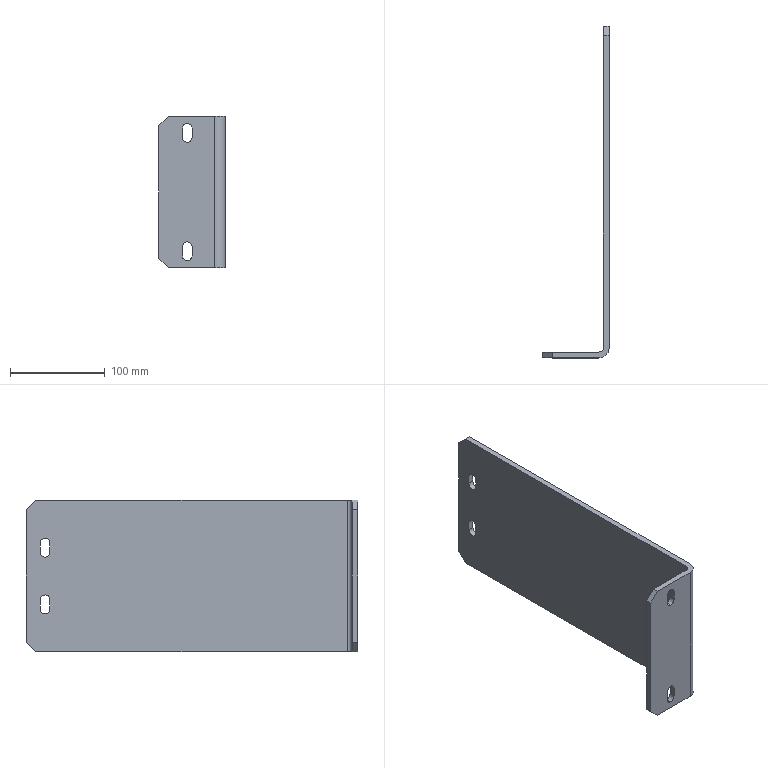Part | STEP file | VD-SYL0380DJ1006_1-1_VD-SYL0380 | 1 solid | 34 faces | box 70 x 350 x 160 mm | volume 388659 mm3 | plane 20 | cylinder 14 | commonest cylinder face diameters 10 x13 22 x1
STEP:
#1=CARTESIAN_POINT('',(0.,325.,35.));
#2=VERTEX_POINT('',#1);
#3=CARTESIAN_POINT('',(0.,330.,40.));
#4=VERTEX_POINT('',#3);
#5=CARTESIAN_POINT('',(0.,330.,35.));
#6=DIRECTION('',(-1.,0.,0.));
#7=DIRECTION('',(0.,-1.,0.));
#8=AXIS2_PLACEMENT_3D('',#5,#6,#7);
#9=CIRCLE('',#8,5.);
#10=EDGE_CURVE('',#2,#4,#9,.T.);
#11=ORIENTED_EDGE('',*,*,#10,.F.);
#12=CARTESIAN_POINT('',(-6.,325.,35.));
#13=VERTEX_POINT('',#12);
#14=CARTESIAN_POINT('',(0.,325.,35.));
#15=DIRECTION('',(-1.,0.,0.));
#16=VECTOR('',#15,1000.);
#17=LINE('',#14,#16);
#18=EDGE_CURVE('',#2,#13,#17,.T.);
#19=ORIENTED_EDGE('',*,*,#18,.T.);
#20=CARTESIAN_POINT('',(-6.,330.,40.));
#21=VERTEX_POINT('',#20);
#22=CARTESIAN_POINT('',(-6.,330.,35.));
#23=DIRECTION('',(1.,0.,0.));
#24=DIRECTION('',(0.,0.,1.));
#25=AXIS2_PLACEMENT_3D('',#22,#23,#24);
#26=CIRCLE('',#25,5.);
#27=EDGE_CURVE('',#21,#13,#26,.T.);
#28=ORIENTED_EDGE('',*,*,#27,.F.);
#29=CARTESIAN_POINT('',(-6.,330.,40.));
#30=DIRECTION('',(1.,0.,0.));
#31=VECTOR('',#30,1000.);
#32=LINE('',#29,#31);
#33=EDGE_CURVE('',#21,#4,#32,.T.);
#34=ORIENTED_EDGE('',*,*,#33,.T.);
#35=EDGE_LOOP('',(#11,#19,#28,#34));
#36=FACE_OUTER_BOUND('',#35,.T.);
#37=CARTESIAN_POINT('',(-3.,330.,35.));
#38=DIRECTION('',(-1.,0.,0.));
#39=DIRECTION('',(0.,0.,1.));
#40=AXIS2_PLACEMENT_3D('',#37,#38,#39);
#41=CYLINDRICAL_SURFACE('',#40,5.);
#42=ADVANCED_FACE('',(#36),#41,.F.);
#43=ORIENTED_EDGE('',*,*,#33,.F.);
#44=CARTESIAN_POINT('',(-6.,335.,35.));
#45=VERTEX_POINT('',#44);
#46=CARTESIAN_POINT('',(-6.,330.,35.));
#47=DIRECTION('',(1.,0.,0.));
#48=DIRECTION('',(0.,1.,0.));
#49=AXIS2_PLACEMENT_3D('',#46,#47,#48);
#50=CIRCLE('',#49,5.);
#51=EDGE_CURVE('',#45,#21,#50,.T.);
#52=ORIENTED_EDGE('',*,*,#51,.F.);
#53=CARTESIAN_POINT('',(0.,335.,35.));
#54=VERTEX_POINT('',#53);
#55=CARTESIAN_POINT('',(-6.,335.,35.));
#56=DIRECTION('',(1.,0.,0.));
#57=VECTOR('',#56,1000.);
#58=LINE('',#55,#57);
#59=EDGE_CURVE('',#45,#54,#58,.T.);
#60=ORIENTED_EDGE('',*,*,#59,.T.);
#61=CARTESIAN_POINT('',(0.,330.,35.));
#62=DIRECTION('',(-1.,0.,0.));
#63=DIRECTION('',(0.,0.,1.));
#64=AXIS2_PLACEMENT_3D('',#61,#62,#63);
#65=CIRCLE('',#64,5.);
#66=EDGE_CURVE('',#4,#54,#65,.T.);
#67=ORIENTED_EDGE('',*,*,#66,.F.);
#68=EDGE_LOOP('',(#43,#52,#60,#67));
#69=FACE_OUTER_BOUND('',#68,.T.);
#70=CARTESIAN_POINT('',(-3.,330.,35.));
#71=DIRECTION('',(-1.,0.,0.));
#72=DIRECTION('',(0.,0.,1.));
#73=AXIS2_PLACEMENT_3D('',#70,#71,#72);
#74=CYLINDRICAL_SURFACE('',#73,5.);
#75=ADVANCED_FACE('',(#69),#74,.F.);
#76=CARTESIAN_POINT('',(0.,335.,25.));
#77=VERTEX_POINT('',#76);
#78=CARTESIAN_POINT('',(-6.,335.,25.));
#79=VERTEX_POINT('',#78);
#80=CARTESIAN_POINT('',(0.,335.,25.));
#81=DIRECTION('',(-1.,0.,0.));
#82=VECTOR('',#81,1000.);
#83=LINE('',#80,#82);
#84=EDGE_CURVE('',#77,#79,#83,.T.);
#85=ORIENTED_EDGE('',*,*,#84,.F.);
#86=CARTESIAN_POINT('',(0.,335.,25.));
#87=DIRECTION('',(0.,0.,1.));
#88=VECTOR('',#87,1000.);
#89=LINE('',#86,#88);
#90=EDGE_CURVE('',#77,#54,#89,.T.);
#91=ORIENTED_EDGE('',*,*,#90,.T.);
#92=ORIENTED_EDGE('',*,*,#59,.F.);
#93=CARTESIAN_POINT('',(-6.,335.,25.));
#94=DIRECTION('',(0.,0.,1.));
#95=VECTOR('',#94,1000.);
#96=LINE('',#93,#95);
#97=EDGE_CURVE('',#79,#45,#96,.T.);
#98=ORIENTED_EDGE('',*,*,#97,.F.);
#99=EDGE_LOOP('',(#85,#91,#92,#98));
#100=FACE_OUTER_BOUND('',#99,.T.);
#101=CARTESIAN_POINT('',(-3.,335.,30.));
#102=DIRECTION('',(0.,1.,0.));
#103=DIRECTION('',(1.,0.,0.));
#104=AXIS2_PLACEMENT_3D('',#101,#102,#103);
#105=PLANE('',#104);
#106=ADVANCED_FACE('',(#100),#105,.F.);
#107=CARTESIAN_POINT('',(-6.,325.,25.));
#108=VERTEX_POINT('',#107);
#109=CARTESIAN_POINT('',(-6.,330.,25.));
#110=DIRECTION('',(1.,0.,0.));
#111=DIRECTION('',(0.,0.,-1.));
#112=AXIS2_PLACEMENT_3D('',#109,#110,#111);
#113=CIRCLE('',#112,5.);
#114=EDGE_CURVE('',#108,#79,#113,.T.);
#115=ORIENTED_EDGE('',*,*,#114,.F.);
#116=CARTESIAN_POINT('',(0.,325.,25.));
#117=VERTEX_POINT('',#116);
#118=CARTESIAN_POINT('',(-6.,325.,25.));
#119=DIRECTION('',(1.,0.,0.));
#120=VECTOR('',#119,1000.);
#121=LINE('',#118,#120);
#122=EDGE_CURVE('',#108,#117,#121,.T.);
#123=ORIENTED_EDGE('',*,*,#122,.T.);
#124=CARTESIAN_POINT('',(0.,330.,25.));
#125=DIRECTION('',(-1.,0.,0.));
#126=DIRECTION('',(0.,1.,0.));
#127=AXIS2_PLACEMENT_3D('',#124,#125,#126);
#128=CIRCLE('',#127,5.);
#129=EDGE_CURVE('',#77,#117,#128,.T.);
#130=ORIENTED_EDGE('',*,*,#129,.F.);
#131=ORIENTED_EDGE('',*,*,#84,.T.);
#132=EDGE_LOOP('',(#115,#123,#130,#131));
#133=FACE_OUTER_BOUND('',#132,.T.);
#134=CARTESIAN_POINT('',(-3.,330.,25.));
#135=DIRECTION('',(-1.,0.,0.));
#136=DIRECTION('',(0.,0.,1.));
#137=AXIS2_PLACEMENT_3D('',#134,#135,#136);
#138=CYLINDRICAL_SURFACE('',#137,5.);
#139=ADVANCED_FACE('',(#133),#138,.F.);
#140=ORIENTED_EDGE('',*,*,#18,.F.);
#141=CARTESIAN_POINT('',(0.,325.,35.));
#142=DIRECTION('',(0.,0.,-1.));
#143=VECTOR('',#142,1000.);
#144=LINE('',#141,#143);
#145=EDGE_CURVE('',#2,#117,#144,.T.);
#146=ORIENTED_EDGE('',*,*,#145,.T.);
#147=ORIENTED_EDGE('',*,*,#122,.F.);
#148=CARTESIAN_POINT('',(-6.,325.,35.));
#149=DIRECTION('',(0.,0.,-1.));
#150=VECTOR('',#149,1000.);
#151=LINE('',#148,#150);
#152=EDGE_CURVE('',#13,#108,#151,.T.);
#153=ORIENTED_EDGE('',*,*,#152,.F.);
#154=EDGE_LOOP('',(#140,#146,#147,#153));
#155=FACE_OUTER_BOUND('',#154,.T.);
#156=CARTESIAN_POINT('',(-3.,325.,30.));
#157=DIRECTION('',(0.,-1.,0.));
#158=DIRECTION('',(0.,0.,-1.));
#159=AXIS2_PLACEMENT_3D('',#156,#157,#158);
#160=PLANE('',#159);
#161=ADVANCED_FACE('',(#155),#160,.F.);
#162=CARTESIAN_POINT('',(0.,325.,-25.));
#163=VERTEX_POINT('',#162);
#164=CARTESIAN_POINT('',(-6.,325.,-25.));
#165=VERTEX_POINT('',#164);
#166=CARTESIAN_POINT('',(0.,325.,-25.));
#167=DIRECTION('',(-1.,0.,0.));
#168=VECTOR('',#167,1000.);
#169=LINE('',#166,#168);
#170=EDGE_CURVE('',#163,#165,#169,.T.);
#171=ORIENTED_EDGE('',*,*,#170,.F.);
#172=CARTESIAN_POINT('',(0.,325.,-35.));
#173=VERTEX_POINT('',#172);
#174=CARTESIAN_POINT('',(0.,325.,-25.));
#175=DIRECTION('',(0.,0.,-1.));
#176=VECTOR('',#175,1000.);
#177=LINE('',#174,#176);
#178=EDGE_CURVE('',#163,#173,#177,.T.);
#179=ORIENTED_EDGE('',*,*,#178,.T.);
#180=CARTESIAN_POINT('',(-6.,325.,-35.));
#181=VERTEX_POINT('',#180);
#182=CARTESIAN_POINT('',(-6.,325.,-35.));
#183=DIRECTION('',(1.,0.,0.));
#184=VECTOR('',#183,1000.);
#185=LINE('',#182,#184);
#186=EDGE_CURVE('',#181,#173,#185,.T.);
#187=ORIENTED_EDGE('',*,*,#186,.F.);
#188=CARTESIAN_POINT('',(-6.,325.,-25.));
#189=DIRECTION('',(0.,0.,-1.));
#190=VECTOR('',#189,1000.);
#191=LINE('',#188,#190);
#192=EDGE_CURVE('',#165,#181,#191,.T.);
#193=ORIENTED_EDGE('',*,*,#192,.F.);
#194=EDGE_LOOP('',(#171,#179,#187,#193));
#195=FACE_OUTER_BOUND('',#194,.T.);
#196=CARTESIAN_POINT('',(-3.,325.,-30.));
#197=DIRECTION('',(0.,-1.,0.));
#198=DIRECTION('',(0.,0.,-1.));
#199=AXIS2_PLACEMENT_3D('',#196,#197,#198);
#200=PLANE('',#199);
#201=ADVANCED_FACE('',(#195),#200,.F.);
#202=CARTESIAN_POINT('',(-6.,335.,-35.));
#203=VERTEX_POINT('',#202);
#204=CARTESIAN_POINT('',(-6.,330.,-35.));
#205=DIRECTION('',(1.,0.,0.));
#206=DIRECTION('',(0.,-1.,0.));
#207=AXIS2_PLACEMENT_3D('',#204,#205,#206);
#208=CIRCLE('',#207,5.);
#209=EDGE_CURVE('',#181,#203,#208,.T.);
#210=ORIENTED_EDGE('',*,*,#209,.F.);
#211=ORIENTED_EDGE('',*,*,#186,.T.);
#212=CARTESIAN_POINT('',(0.,335.,-35.));
#213=VERTEX_POINT('',#212);
#214=CARTESIAN_POINT('',(0.,330.,-35.));
#215=DIRECTION('',(-1.,0.,0.));
#216=DIRECTION('',(0.,1.,0.));
#217=AXIS2_PLACEMENT_3D('',#214,#215,#216);
#218=CIRCLE('',#217,5.);
#219=EDGE_CURVE('',#213,#173,#218,.T.);
#220=ORIENTED_EDGE('',*,*,#219,.F.);
#221=CARTESIAN_POINT('',(0.,335.,-35.));
#222=DIRECTION('',(-1.,0.,0.));
#223=VECTOR('',#222,1000.);
#224=LINE('',#221,#223);
#225=EDGE_CURVE('',#213,#203,#224,.T.);
#226=ORIENTED_EDGE('',*,*,#225,.T.);
#227=EDGE_LOOP('',(#210,#211,#220,#226));
#228=FACE_OUTER_BOUND('',#227,.T.);
#229=CARTESIAN_POINT('',(-3.,330.,-35.));
#230=DIRECTION('',(-1.,0.,0.));
#231=DIRECTION('',(0.,0.,1.));
#232=AXIS2_PLACEMENT_3D('',#229,#230,#231);
#233=CYLINDRICAL_SURFACE('',#232,5.);
#234=ADVANCED_FACE('',(#228),#233,.F.);
#235=ORIENTED_EDGE('',*,*,#225,.F.);
#236=CARTESIAN_POINT('',(0.,335.,-25.));
#237=VERTEX_POINT('',#236);
#238=CARTESIAN_POINT('',(0.,335.,-35.));
#239=DIRECTION('',(0.,0.,1.));
#240=VECTOR('',#239,1000.);
#241=LINE('',#238,#240);
#242=EDGE_CURVE('',#213,#237,#241,.T.);
#243=ORIENTED_EDGE('',*,*,#242,.T.);
#244=CARTESIAN_POINT('',(-6.,335.,-25.));
#245=VERTEX_POINT('',#244);
#246=CARTESIAN_POINT('',(-6.,335.,-25.));
#247=DIRECTION('',(1.,0.,0.));
#248=VECTOR('',#247,1000.);
#249=LINE('',#246,#248);
#250=EDGE_CURVE('',#245,#237,#249,.T.);
#251=ORIENTED_EDGE('',*,*,#250,.F.);
#252=CARTESIAN_POINT('',(-6.,335.,-35.));
#253=DIRECTION('',(0.,0.,1.));
#254=VECTOR('',#253,1000.);
#255=LINE('',#252,#254);
#256=EDGE_CURVE('',#203,#245,#255,.T.);
#257=ORIENTED_EDGE('',*,*,#256,.F.);
#258=EDGE_LOOP('',(#235,#243,#251,#257));
#259=FACE_OUTER_BOUND('',#258,.T.);
#260=CARTESIAN_POINT('',(-3.,335.,-30.));
#261=DIRECTION('',(0.,1.,0.));
#262=DIRECTION('',(1.,0.,0.));
#263=AXIS2_PLACEMENT_3D('',#260,#261,#262);
#264=PLANE('',#263);
#265=ADVANCED_FACE('',(#259),#264,.F.);
#266=CARTESIAN_POINT('',(-6.,330.,-20.));
#267=VERTEX_POINT('',#266);
#268=CARTESIAN_POINT('',(0.,330.,-20.));
#269=VERTEX_POINT('',#268);
#270=CARTESIAN_POINT('',(-6.,330.,-20.));
#271=DIRECTION('',(1.,0.,0.));
#272=VECTOR('',#271,1000.);
#273=LINE('',#270,#272);
#274=EDGE_CURVE('',#267,#269,#273,.T.);
#275=ORIENTED_EDGE('',*,*,#274,.F.);
#276=CARTESIAN_POINT('',(-6.,330.,-25.));
#277=DIRECTION('',(1.,0.,0.));
#278=DIRECTION('',(0.,1.,0.));
#279=AXIS2_PLACEMENT_3D('',#276,#277,#278);
#280=CIRCLE('',#279,5.);
#281=EDGE_CURVE('',#245,#267,#280,.T.);
#282=ORIENTED_EDGE('',*,*,#281,.F.);
#283=ORIENTED_EDGE('',*,*,#250,.T.);
#284=CARTESIAN_POINT('',(0.,330.,-25.));
#285=DIRECTION('',(-1.,0.,0.));
#286=DIRECTION('',(0.,0.,1.));
#287=AXIS2_PLACEMENT_3D('',#284,#285,#286);
#288=CIRCLE('',#287,5.);
#289=EDGE_CURVE('',#269,#237,#288,.T.);
#290=ORIENTED_EDGE('',*,*,#289,.F.);
#291=EDGE_LOOP('',(#275,#282,#283,#290));
#292=FACE_OUTER_BOUND('',#291,.T.);
#293=CARTESIAN_POINT('',(-3.,330.,-25.));
#294=DIRECTION('',(-1.,0.,0.));
#295=DIRECTION('',(0.,0.,1.));
#296=AXIS2_PLACEMENT_3D('',#293,#294,#295);
#297=CYLINDRICAL_SURFACE('',#296,5.);
#298=ADVANCED_FACE('',(#292),#297,.F.);
#299=CARTESIAN_POINT('',(0.,330.,-25.));
#300=DIRECTION('',(-1.,0.,0.));
#301=DIRECTION('',(0.,-1.,0.));
#302=AXIS2_PLACEMENT_3D('',#299,#300,#301);
#303=CIRCLE('',#302,5.);
#304=EDGE_CURVE('',#163,#269,#303,.T.);
#305=ORIENTED_EDGE('',*,*,#304,.F.);
#306=ORIENTED_EDGE('',*,*,#170,.T.);
#307=CARTESIAN_POINT('',(-6.,330.,-25.));
#308=DIRECTION('',(1.,0.,0.));
#309=DIRECTION('',(0.,0.,1.));
#310=AXIS2_PLACEMENT_3D('',#307,#308,#309);
#311=CIRCLE('',#310,5.);
#312=EDGE_CURVE('',#267,#165,#311,.T.);
#313=ORIENTED_EDGE('',*,*,#312,.F.);
#314=ORIENTED_EDGE('',*,*,#274,.T.);
#315=EDGE_LOOP('',(#305,#306,#313,#314));
#316=FACE_OUTER_BOUND('',#315,.T.);
#317=CARTESIAN_POINT('',(-3.,330.,-25.));
#318=DIRECTION('',(-1.,0.,0.));
#319=DIRECTION('',(0.,0.,1.));
#320=AXIS2_PLACEMENT_3D('',#317,#318,#319);
#321=CYLINDRICAL_SURFACE('',#320,5.);
#322=ADVANCED_FACE('',(#316),#321,.F.);
#323=CARTESIAN_POINT('',(0.,340.,-80.));
#324=VERTEX_POINT('',#323);
#325=CARTESIAN_POINT('',(0.,350.,-70.));
#326=VERTEX_POINT('',#325);
#327=CARTESIAN_POINT('',(0.,340.,-80.));
#328=DIRECTION('',(0.,0.7071,0.7071));
#329=VECTOR('',#328,1000.);
#330=LINE('',#327,#329);
#331=EDGE_CURVE('',#324,#326,#330,.T.);
#332=ORIENTED_EDGE('',*,*,#331,.F.);
#333=CARTESIAN_POINT('',(-6.,340.,-80.));
#334=VERTEX_POINT('',#333);
#335=CARTESIAN_POINT('',(0.,340.,-80.));
#336=DIRECTION('',(-1.,0.,0.));
#337=VECTOR('',#336,1000.);
#338=LINE('',#335,#337);
#339=EDGE_CURVE('',#324,#334,#338,.T.);
#340=ORIENTED_EDGE('',*,*,#339,.T.);
#341=CARTESIAN_POINT('',(-6.,350.,-70.));
#342=VERTEX_POINT('',#341);
#343=CARTESIAN_POINT('',(-6.,350.,-70.));
#344=DIRECTION('',(0.,-0.7071,-0.7071));
#345=VECTOR('',#344,1000.);
#346=LINE('',#343,#345);
#347=EDGE_CURVE('',#342,#334,#346,.T.);
#348=ORIENTED_EDGE('',*,*,#347,.F.);
#349=CARTESIAN_POINT('',(-6.,350.,-70.));
#350=DIRECTION('',(1.,0.,0.));
#351=VECTOR('',#350,1000.);
#352=LINE('',#349,#351);
#353=EDGE_CURVE('',#342,#326,#352,.T.);
#354=ORIENTED_EDGE('',*,*,#353,.T.);
#355=EDGE_LOOP('',(#332,#340,#348,#354));
#356=FACE_OUTER_BOUND('',#355,.T.);
#357=CARTESIAN_POINT('',(-3.,345.,-75.));
#358=DIRECTION('',(0.,0.7071,-0.7071));
#359=DIRECTION('',(-1.,0.,0.));
#360=AXIS2_PLACEMENT_3D('',#357,#358,#359);
#361=PLANE('',#360);
#362=ADVANCED_FACE('',(#356),#361,.T.);
#363=CARTESIAN_POINT('',(-45.,6.,57.5));
#364=VERTEX_POINT('',#363);
#365=CARTESIAN_POINT('',(-40.,6.,52.5));
#366=VERTEX_POINT('',#365);
#367=CARTESIAN_POINT('',(-40.,6.,57.5));
#368=DIRECTION('',(0.,-1.,0.));
#369=DIRECTION('',(-1.,0.,0.));
#370=AXIS2_PLACEMENT_3D('',#367,#368,#369);
#371=CIRCLE('',#370,5.);
#372=EDGE_CURVE('',#364,#366,#371,.T.);
#373=ORIENTED_EDGE('',*,*,#372,.F.);
#374=CARTESIAN_POINT('',(-45.,0.,57.5));
#375=VERTEX_POINT('',#374);
#376=CARTESIAN_POINT('',(-45.,6.,57.5));
#377=DIRECTION('',(0.,-1.,0.));
#378=VECTOR('',#377,1000.);
#379=LINE('',#376,#378);
#380=EDGE_CURVE('',#364,#375,#379,.T.);
#381=ORIENTED_EDGE('',*,*,#380,.T.);
#382=CARTESIAN_POINT('',(-40.,0.,52.5));
#383=VERTEX_POINT('',#382);
#384=CARTESIAN_POINT('',(-40.,0.,57.5));
#385=DIRECTION('',(0.,1.,0.));
#386=DIRECTION('',(0.,0.,-1.));
#387=AXIS2_PLACEMENT_3D('',#384,#385,#386);
#388=CIRCLE('',#387,5.);
#389=EDGE_CURVE('',#383,#375,#388,.T.);
#390=ORIENTED_EDGE('',*,*,#389,.F.);
#391=CARTESIAN_POINT('',(-40.,0.,52.5));
#392=DIRECTION('',(0.,1.,0.));
#393=VECTOR('',#392,1000.);
#394=LINE('',#391,#393);
#395=EDGE_CURVE('',#383,#366,#394,.T.);
#396=ORIENTED_EDGE('',*,*,#395,.T.);
#397=EDGE_LOOP('',(#373,#381,#390,#396));
#398=FACE_OUTER_BOUND('',#397,.T.);
#399=CARTESIAN_POINT('',(-40.,3.,57.5));
#400=DIRECTION('',(0.,-1.,0.));
#401=DIRECTION('',(0.,0.,-1.));
#402=AXIS2_PLACEMENT_3D('',#399,#400,#401);
#403=CYLINDRICAL_SURFACE('',#402,5.);
#404=ADVANCED_FACE('',(#398),#403,.F.);
#405=CARTESIAN_POINT('',(-35.,0.,67.5));
#406=VERTEX_POINT('',#405);
#407=CARTESIAN_POINT('',(-35.,0.,57.5));
#408=VERTEX_POINT('',#407);
#409=CARTESIAN_POINT('',(-35.,0.,67.5));
#410=DIRECTION('',(0.,0.,-1.));
#411=VECTOR('',#410,1000.);
#412=LINE('',#409,#411);
#413=EDGE_CURVE('',#406,#408,#412,.T.);
#414=ORIENTED_EDGE('',*,*,#413,.F.);
#415=CARTESIAN_POINT('',(-35.,6.,67.5));
#416=VERTEX_POINT('',#415);
#417=CARTESIAN_POINT('',(-35.,6.,67.5));
#418=DIRECTION('',(0.,-1.,0.));
#419=VECTOR('',#418,1000.);
#420=LINE('',#417,#419);
#421=EDGE_CURVE('',#416,#406,#420,.T.);
#422=ORIENTED_EDGE('',*,*,#421,.F.);
#423=CARTESIAN_POINT('',(-35.,6.,57.5));
#424=VERTEX_POINT('',#423);
#425=CARTESIAN_POINT('',(-35.,6.,57.5));
#426=DIRECTION('',(0.,0.,1.));
#427=VECTOR('',#426,1000.);
#428=LINE('',#425,#427);
#429=EDGE_CURVE('',#424,#416,#428,.T.);
#430=ORIENTED_EDGE('',*,*,#429,.F.);
#431=CARTESIAN_POINT('',(-35.,0.,57.5));
#432=DIRECTION('',(0.,1.,0.));
#433=VECTOR('',#432,1000.);
#434=LINE('',#431,#433);
#435=EDGE_CURVE('',#408,#424,#434,.T.);
#436=ORIENTED_EDGE('',*,*,#435,.F.);
#437=EDGE_LOOP('',(#414,#422,#430,#436));
#438=FACE_OUTER_BOUND('',#437,.T.);
#439=CARTESIAN_POINT('',(-35.,3.,62.5));
#440=DIRECTION('',(-1.,0.,0.));
#441=DIRECTION('',(0.,0.,1.));
#442=AXIS2_PLACEMENT_3D('',#439,#440,#441);
#443=PLANE('',#442);
#444=ADVANCED_FACE('',(#438),#443,.T.);
#445=CARTESIAN_POINT('',(-45.,6.,67.5));
#446=VERTEX_POINT('',#445);
#447=CARTESIAN_POINT('',(-40.,6.,67.5));
#448=DIRECTION('',(0.,-1.,0.));
#449=DIRECTION('',(1.,0.,0.));
#450=AXIS2_PLACEMENT_3D('',#447,#448,#449);
#451=CIRCLE('',#450,5.);
#452=EDGE_CURVE('',#416,#446,#451,.T.);
#453=ORIENTED_EDGE('',*,*,#452,.F.);
#454=ORIENTED_EDGE('',*,*,#421,.T.);
#455=CARTESIAN_POINT('',(-45.,0.,67.5));
#456=VERTEX_POINT('',#455);
#457=CARTESIAN_POINT('',(-40.,0.,67.5));
#458=DIRECTION('',(0.,1.,0.));
#459=DIRECTION('',(-1.,0.,0.));
#460=AXIS2_PLACEMENT_3D('',#457,#458,#459);
#461=CIRCLE('',#460,5.);
#462=EDGE_CURVE('',#456,#406,#461,.T.);
#463=ORIENTED_EDGE('',*,*,#462,.F.);
#464=CARTESIAN_POINT('',(-45.,0.,67.5));
#465=DIRECTION('',(0.,1.,0.));
#466=VECTOR('',#465,1000.);
#467=LINE('',#464,#466);
#468=EDGE_CURVE('',#456,#446,#467,.T.);
#469=ORIENTED_EDGE('',*,*,#468,.T.);
#470=EDGE_LOOP('',(#453,#454,#463,#469));
#471=FACE_OUTER_BOUND('',#470,.T.);
#472=CARTESIAN_POINT('',(-40.,3.,67.5));
#473=DIRECTION('',(0.,-1.,0.));
#474=DIRECTION('',(0.,0.,-1.));
#475=AXIS2_PLACEMENT_3D('',#472,#473,#474);
#476=CYLINDRICAL_SURFACE('',#475,5.);
#477=ADVANCED_FACE('',(#471),#476,.F.);
#478=CARTESIAN_POINT('',(-45.,0.,57.5));
#479=DIRECTION('',(0.,0.,1.));
#480=VECTOR('',#479,1000.);
#481=LINE('',#478,#480);
#482=EDGE_CURVE('',#375,#456,#481,.T.);
#483=ORIENTED_EDGE('',*,*,#482,.F.);
#484=ORIENTED_EDGE('',*,*,#380,.F.);
#485=CARTESIAN_POINT('',(-45.,6.,67.5));
#486=DIRECTION('',(0.,0.,-1.));
#487=VECTOR('',#486,1000.);
#488=LINE('',#485,#487);
#489=EDGE_CURVE('',#446,#364,#488,.T.);
#490=ORIENTED_EDGE('',*,*,#489,.F.);
#491=ORIENTED_EDGE('',*,*,#468,.F.);
#492=EDGE_LOOP('',(#483,#484,#490,#491));
#493=FACE_OUTER_BOUND('',#492,.T.);
#494=CARTESIAN_POINT('',(-45.,3.,62.5));
#495=DIRECTION('',(1.,0.,0.));
#496=DIRECTION('',(0.,1.,0.));
#497=AXIS2_PLACEMENT_3D('',#494,#495,#496);
#498=PLANE('',#497);
#499=ADVANCED_FACE('',(#493),#498,.T.);
#500=CARTESIAN_POINT('',(-45.,6.,-67.5));
#501=VERTEX_POINT('',#500);
#502=CARTESIAN_POINT('',(-40.,6.,-72.5));
#503=VERTEX_POINT('',#502);
#504=CARTESIAN_POINT('',(-40.,6.,-67.5));
#505=DIRECTION('',(0.,-1.,0.));
#506=DIRECTION('',(-1.,0.,0.));
#507=AXIS2_PLACEMENT_3D('',#504,#505,#506);
#508=CIRCLE('',#507,5.);
#509=EDGE_CURVE('',#501,#503,#508,.T.);
#510=ORIENTED_EDGE('',*,*,#509,.F.);
#511=CARTESIAN_POINT('',(-45.,0.,-67.5));
#512=VERTEX_POINT('',#511);
#513=CARTESIAN_POINT('',(-45.,6.,-67.5));
#514=DIRECTION('',(0.,-1.,0.));
#515=VECTOR('',#514,1000.);
#516=LINE('',#513,#515);
#517=EDGE_CURVE('',#501,#512,#516,.T.);
#518=ORIENTED_EDGE('',*,*,#517,.T.);
#519=CARTESIAN_POINT('',(-40.,0.,-72.5));
#520=VERTEX_POINT('',#519);
#521=CARTESIAN_POINT('',(-40.,0.,-67.5));
#522=DIRECTION('',(0.,1.,0.));
#523=DIRECTION('',(0.,0.,-1.));
#524=AXIS2_PLACEMENT_3D('',#521,#522,#523);
#525=CIRCLE('',#524,5.);
#526=EDGE_CURVE('',#520,#512,#525,.T.);
#527=ORIENTED_EDGE('',*,*,#526,.F.);
#528=CARTESIAN_POINT('',(-40.,0.,-72.5));
#529=DIRECTION('',(0.,1.,0.));
#530=VECTOR('',#529,1000.);
#531=LINE('',#528,#530);
#532=EDGE_CURVE('',#520,#503,#531,.T.);
#533=ORIENTED_EDGE('',*,*,#532,.T.);
#534=EDGE_LOOP('',(#510,#518,#527,#533));
#535=FACE_OUTER_BOUND('',#534,.T.);
#536=CARTESIAN_POINT('',(-40.,3.,-67.5));
#537=DIRECTION('',(0.,-1.,0.));
#538=DIRECTION('',(0.,0.,-1.));
#539=AXIS2_PLACEMENT_3D('',#536,#537,#538);
#540=CYLINDRICAL_SURFACE('',#539,5.);
#541=ADVANCED_FACE('',(#535),#540,.F.);
#542=CARTESIAN_POINT('',(-45.,0.,-57.5));
#543=VERTEX_POINT('',#542);
#544=CARTESIAN_POINT('',(-45.,0.,-67.5));
#545=DIRECTION('',(0.,0.,1.));
#546=VECTOR('',#545,1000.);
#547=LINE('',#544,#546);
#548=EDGE_CURVE('',#512,#543,#547,.T.);
#549=ORIENTED_EDGE('',*,*,#548,.F.);
#550=ORIENTED_EDGE('',*,*,#517,.F.);
#551=CARTESIAN_POINT('',(-45.,6.,-57.5));
#552=VERTEX_POINT('',#551);
#553=CARTESIAN_POINT('',(-45.,6.,-57.5));
#554=DIRECTION('',(0.,0.,-1.));
#555=VECTOR('',#554,1000.);
#556=LINE('',#553,#555);
#557=EDGE_CURVE('',#552,#501,#556,.T.);
#558=ORIENTED_EDGE('',*,*,#557,.F.);
#559=CARTESIAN_POINT('',(-45.,0.,-57.5));
#560=DIRECTION('',(0.,1.,0.));
#561=VECTOR('',#560,1000.);
#562=LINE('',#559,#561);
#563=EDGE_CURVE('',#543,#552,#562,.T.);
#564=ORIENTED_EDGE('',*,*,#563,.F.);
#565=EDGE_LOOP('',(#549,#550,#558,#564));
#566=FACE_OUTER_BOUND('',#565,.T.);
#567=CARTESIAN_POINT('',(-45.,3.,-62.5));
#568=DIRECTION('',(1.,0.,0.));
#569=DIRECTION('',(0.,1.,0.));
#570=AXIS2_PLACEMENT_3D('',#567,#568,#569);
#571=PLANE('',#570);
#572=ADVANCED_FACE('',(#566),#571,.T.);
#573=CARTESIAN_POINT('',(-35.,6.,-57.5));
#574=VERTEX_POINT('',#573);
#575=CARTESIAN_POINT('',(-40.,6.,-57.5));
#576=DIRECTION('',(0.,-1.,0.));
#577=DIRECTION('',(1.,0.,0.));
#578=AXIS2_PLACEMENT_3D('',#575,#576,#577);
#579=CIRCLE('',#578,5.);
#580=EDGE_CURVE('',#574,#552,#579,.T.);
#581=ORIENTED_EDGE('',*,*,#580,.F.);
#582=CARTESIAN_POINT('',(-35.,0.,-57.5));
#583=VERTEX_POINT('',#582);
#584=CARTESIAN_POINT('',(-35.,6.,-57.5));
#585=DIRECTION('',(0.,-1.,0.));
#586=VECTOR('',#585,1000.);
#587=LINE('',#584,#586);
#588=EDGE_CURVE('',#574,#583,#587,.T.);
#589=ORIENTED_EDGE('',*,*,#588,.T.);
#590=CARTESIAN_POINT('',(-40.,0.,-57.5));
#591=DIRECTION('',(0.,1.,0.));
#592=DIRECTION('',(-1.,0.,0.));
#593=AXIS2_PLACEMENT_3D('',#590,#591,#592);
#594=CIRCLE('',#593,5.);
#595=EDGE_CURVE('',#543,#583,#594,.T.);
#596=ORIENTED_EDGE('',*,*,#595,.F.);
#597=ORIENTED_EDGE('',*,*,#563,.T.);
#598=EDGE_LOOP('',(#581,#589,#596,#597));
#599=FACE_OUTER_BOUND('',#598,.T.);
#600=CARTESIAN_POINT('',(-40.,3.,-57.5));
#601=DIRECTION('',(0.,-1.,0.));
#602=DIRECTION('',(0.,0.,-1.));
#603=AXIS2_PLACEMENT_3D('',#600,#601,#602);
#604=CYLINDRICAL_SURFACE('',#603,5.);
#605=ADVANCED_FACE('',(#599),#604,.F.);
#606=CARTESIAN_POINT('',(-35.,0.,-67.5));
#607=VERTEX_POINT('',#606);
#608=CARTESIAN_POINT('',(-35.,0.,-57.5));
#609=DIRECTION('',(0.,0.,-1.));
#610=VECTOR('',#609,1000.);
#611=LINE('',#608,#610);
#612=EDGE_CURVE('',#583,#607,#611,.T.);
#613=ORIENTED_EDGE('',*,*,#612,.F.);
#614=ORIENTED_EDGE('',*,*,#588,.F.);
#615=CARTESIAN_POINT('',(-35.,6.,-67.5));
#616=VERTEX_POINT('',#615);
#617=CARTESIAN_POINT('',(-35.,6.,-67.5));
#618=DIRECTION('',(0.,0.,1.));
#619=VECTOR('',#618,1000.);
#620=LINE('',#617,#619);
#621=EDGE_CURVE('',#616,#574,#620,.T.);
#622=ORIENTED_EDGE('',*,*,#621,.F.);
#623=CARTESIAN_POINT('',(-35.,0.,-67.5));
#624=DIRECTION('',(0.,1.,0.));
#625=VECTOR('',#624,1000.);
#626=LINE('',#623,#625);
#627=EDGE_CURVE('',#607,#616,#626,.T.);
#628=ORIENTED_EDGE('',*,*,#627,.F.);
#629=EDGE_LOOP('',(#613,#614,#622,#628));
#630=FACE_OUTER_BOUND('',#629,.T.);
#631=CARTESIAN_POINT('',(-35.,3.,-62.5));
#632=DIRECTION('',(-1.,0.,0.));
#633=DIRECTION('',(0.,0.,1.));
#634=AXIS2_PLACEMENT_3D('',#631,#632,#633);
#635=PLANE('',#634);
#636=ADVANCED_FACE('',(#630),#635,.T.);
#637=ORIENTED_EDGE('',*,*,#532,.F.);
#638=CARTESIAN_POINT('',(-40.,0.,-67.5));
#639=DIRECTION('',(0.,1.,0.));
#640=DIRECTION('',(1.,0.,0.));
#641=AXIS2_PLACEMENT_3D('',#638,#639,#640);
#642=CIRCLE('',#641,5.);
#643=EDGE_CURVE('',#607,#520,#642,.T.);
#644=ORIENTED_EDGE('',*,*,#643,.F.);
#645=ORIENTED_EDGE('',*,*,#627,.T.);
#646=CARTESIAN_POINT('',(-40.,6.,-67.5));
#647=DIRECTION('',(0.,-1.,0.));
#648=DIRECTION('',(0.,0.,-1.));
#649=AXIS2_PLACEMENT_3D('',#646,#647,#648);
#650=CIRCLE('',#649,5.);
#651=EDGE_CURVE('',#503,#616,#650,.T.);
#652=ORIENTED_EDGE('',*,*,#651,.F.);
#653=EDGE_LOOP('',(#637,#644,#645,#652));
#654=FACE_OUTER_BOUND('',#653,.T.);
#655=CARTESIAN_POINT('',(-40.,3.,-67.5));
#656=DIRECTION('',(0.,-1.,0.));
#657=DIRECTION('',(0.,0.,-1.));
#658=AXIS2_PLACEMENT_3D('',#655,#656,#657);
#659=CYLINDRICAL_SURFACE('',#658,5.);
#660=ADVANCED_FACE('',(#654),#659,.F.);
#661=ORIENTED_EDGE('',*,*,#462,.T.);
#662=ORIENTED_EDGE('',*,*,#413,.T.);
#663=CARTESIAN_POINT('',(-40.,0.,57.5));
#664=DIRECTION('',(0.,1.,0.));
#665=DIRECTION('',(1.,0.,0.));
#666=AXIS2_PLACEMENT_3D('',#663,#664,#665);
#667=CIRCLE('',#666,5.);
#668=EDGE_CURVE('',#408,#383,#667,.T.);
#669=ORIENTED_EDGE('',*,*,#668,.T.);
#670=ORIENTED_EDGE('',*,*,#389,.T.);
#671=ORIENTED_EDGE('',*,*,#482,.T.);
#672=EDGE_LOOP('',(#661,#662,#669,#670,#671));
#673=FACE_BOUND('',#672,.T.);
#674=ORIENTED_EDGE('',*,*,#526,.T.);
#675=ORIENTED_EDGE('',*,*,#548,.T.);
#676=ORIENTED_EDGE('',*,*,#595,.T.);
#677=ORIENTED_EDGE('',*,*,#612,.T.);
#678=ORIENTED_EDGE('',*,*,#643,.T.);
#679=EDGE_LOOP('',(#674,#675,#676,#677,#678));
#680=FACE_BOUND('',#679,.T.);
#681=CARTESIAN_POINT('',(-60.,0.,80.));
#682=VERTEX_POINT('',#681);
#683=CARTESIAN_POINT('',(-70.,0.,70.));
#684=VERTEX_POINT('',#683);
#685=CARTESIAN_POINT('',(-60.,0.,80.));
#686=DIRECTION('',(-0.7071,0.,-0.7071));
#687=VECTOR('',#686,1000.);
#688=LINE('',#685,#687);
#689=EDGE_CURVE('',#682,#684,#688,.T.);
#690=ORIENTED_EDGE('',*,*,#689,.T.);
#691=CARTESIAN_POINT('',(-70.,0.,-70.));
#692=VERTEX_POINT('',#691);
#693=CARTESIAN_POINT('',(-70.,0.,-70.));
#694=DIRECTION('',(0.,0.,1.));
#695=VECTOR('',#694,1000.);
#696=LINE('',#693,#695);
#697=EDGE_CURVE('',#692,#684,#696,.T.);
#698=ORIENTED_EDGE('',*,*,#697,.F.);
#699=CARTESIAN_POINT('',(-60.,0.,-80.));
#700=VERTEX_POINT('',#699);
#701=CARTESIAN_POINT('',(-70.,0.,-70.));
#702=DIRECTION('',(0.7071,0.,-0.7071));
#703=VECTOR('',#702,1000.);
#704=LINE('',#701,#703);
#705=EDGE_CURVE('',#692,#700,#704,.T.);
#706=ORIENTED_EDGE('',*,*,#705,.T.);
#707=CARTESIAN_POINT('',(-11.,0.,-80.));
#708=VERTEX_POINT('',#707);
#709=CARTESIAN_POINT('',(-60.,0.,-80.));
#710=DIRECTION('',(1.,0.,0.));
#711=VECTOR('',#710,1000.);
#712=LINE('',#709,#711);
#713=EDGE_CURVE('',#700,#708,#712,.T.);
#714=ORIENTED_EDGE('',*,*,#713,.T.);
#715=CARTESIAN_POINT('',(-11.,0.,80.));
#716=VERTEX_POINT('',#715);
#717=CARTESIAN_POINT('',(-11.,0.,80.));
#718=DIRECTION('',(0.,0.,-1.));
#719=VECTOR('',#718,1000.);
#720=LINE('',#717,#719);
#721=EDGE_CURVE('',#716,#708,#720,.T.);
#722=ORIENTED_EDGE('',*,*,#721,.F.);
#723=CARTESIAN_POINT('',(-60.,0.,80.));
#724=DIRECTION('',(1.,0.,0.));
#725=VECTOR('',#724,1000.);
#726=LINE('',#723,#725);
#727=EDGE_CURVE('',#682,#716,#726,.T.);
#728=ORIENTED_EDGE('',*,*,#727,.F.);
#729=EDGE_LOOP('',(#690,#698,#706,#714,#722,#728));
#730=FACE_OUTER_BOUND('',#729,.T.);
#731=CARTESIAN_POINT('',(-70.,0.,-80.));
#732=DIRECTION('',(0.,-1.,0.));
#733=DIRECTION('',(0.,0.,-1.));
#734=AXIS2_PLACEMENT_3D('',#731,#732,#733);
#735=PLANE('',#734);
#736=ADVANCED_FACE('',(#673,#680,#730),#735,.T.);
#737=ORIENTED_EDGE('',*,*,#721,.T.);
#738=CARTESIAN_POINT('',(0.,11.,-80.));
#739=VERTEX_POINT('',#738);
#740=CARTESIAN_POINT('',(-11.,11.,-80.));
#741=DIRECTION('',(0.,0.,-1.));
#742=DIRECTION('',(1.,0.,0.));
#743=AXIS2_PLACEMENT_3D('',#740,#741,#742);
#744=CIRCLE('',#743,11.);
#745=EDGE_CURVE('',#739,#708,#744,.T.);
#746=ORIENTED_EDGE('',*,*,#745,.F.);
#747=CARTESIAN_POINT('',(0.,11.,80.));
#748=VERTEX_POINT('',#747);
#749=CARTESIAN_POINT('',(0.,11.,-80.));
#750=DIRECTION('',(0.,0.,1.));
#751=VECTOR('',#750,1000.);
#752=LINE('',#749,#751);
#753=EDGE_CURVE('',#739,#748,#752,.T.);
#754=ORIENTED_EDGE('',*,*,#753,.T.);
#755=CARTESIAN_POINT('',(-11.,11.,80.));
#756=DIRECTION('',(0.,0.,1.));
#757=DIRECTION('',(0.,-1.,0.));
#758=AXIS2_PLACEMENT_3D('',#755,#756,#757);
#759=CIRCLE('',#758,11.);
#760=EDGE_CURVE('',#716,#748,#759,.T.);
#761=ORIENTED_EDGE('',*,*,#760,.F.);
#762=EDGE_LOOP('',(#737,#746,#754,#761));
#763=FACE_OUTER_BOUND('',#762,.T.);
#764=CARTESIAN_POINT('',(-11.,11.,408.843));
#765=DIRECTION('',(0.,0.,-1.));
#766=DIRECTION('',(-1.,0.,0.));
#767=AXIS2_PLACEMENT_3D('',#764,#765,#766);
#768=CYLINDRICAL_SURFACE('',#767,11.);
#769=ADVANCED_FACE('',(#763),#768,.T.);
#770=ORIENTED_EDGE('',*,*,#10,.T.);
#771=ORIENTED_EDGE('',*,*,#66,.T.);
#772=ORIENTED_EDGE('',*,*,#90,.F.);
#773=ORIENTED_EDGE('',*,*,#129,.T.);
#774=ORIENTED_EDGE('',*,*,#145,.F.);
#775=EDGE_LOOP('',(#770,#771,#772,#773,#774));
#776=FACE_BOUND('',#775,.T.);
#777=ORIENTED_EDGE('',*,*,#289,.T.);
#778=ORIENTED_EDGE('',*,*,#242,.F.);
#779=ORIENTED_EDGE('',*,*,#219,.T.);
#780=ORIENTED_EDGE('',*,*,#178,.F.);
#781=ORIENTED_EDGE('',*,*,#304,.T.);
#782=EDGE_LOOP('',(#777,#778,#779,#780,#781));
#783=FACE_BOUND('',#782,.T.);
#784=ORIENTED_EDGE('',*,*,#331,.T.);
#785=CARTESIAN_POINT('',(0.,350.,70.));
#786=VERTEX_POINT('',#785);
#787=CARTESIAN_POINT('',(0.,350.,-70.));
#788=DIRECTION('',(0.,0.,1.));
#789=VECTOR('',#788,1000.);
#790=LINE('',#787,#789);
#791=EDGE_CURVE('',#326,#786,#790,.T.);
#792=ORIENTED_EDGE('',*,*,#791,.T.);
#793=CARTESIAN_POINT('',(0.,340.,80.));
#794=VERTEX_POINT('',#793);
#795=CARTESIAN_POINT('',(0.,350.,70.));
#796=DIRECTION('',(0.,-0.7071,0.7071));
#797=VECTOR('',#796,1000.);
#798=LINE('',#795,#797);
#799=EDGE_CURVE('',#786,#794,#798,.T.);
#800=ORIENTED_EDGE('',*,*,#799,.T.);
#801=CARTESIAN_POINT('',(0.,11.,80.));
#802=DIRECTION('',(0.,1.,0.));
#803=VECTOR('',#802,1000.);
#804=LINE('',#801,#803);
#805=EDGE_CURVE('',#748,#794,#804,.T.);
#806=ORIENTED_EDGE('',*,*,#805,.F.);
#807=ORIENTED_EDGE('',*,*,#753,.F.);
#808=CARTESIAN_POINT('',(0.,11.,-80.));
#809=DIRECTION('',(0.,1.,0.));
#810=VECTOR('',#809,1000.);
#811=LINE('',#808,#810);
#812=EDGE_CURVE('',#739,#324,#811,.T.);
#813=ORIENTED_EDGE('',*,*,#812,.T.);
#814=EDGE_LOOP('',(#784,#792,#800,#806,#807,#813));
#815=FACE_OUTER_BOUND('',#814,.T.);
#816=CARTESIAN_POINT('',(0.,0.,-80.));
#817=DIRECTION('',(1.,0.,0.));
#818=DIRECTION('',(0.,1.,0.));
#819=AXIS2_PLACEMENT_3D('',#816,#817,#818);
#820=PLANE('',#819);
#821=ADVANCED_FACE('',(#776,#783,#815),#820,.T.);
#822=ORIENTED_EDGE('',*,*,#353,.F.);
#823=CARTESIAN_POINT('',(-6.,350.,70.));
#824=VERTEX_POINT('',#823);
#825=CARTESIAN_POINT('',(-6.,350.,70.));
#826=DIRECTION('',(0.,0.,-1.));
#827=VECTOR('',#826,1000.);
#828=LINE('',#825,#827);
#829=EDGE_CURVE('',#824,#342,#828,.T.);
#830=ORIENTED_EDGE('',*,*,#829,.F.);
#831=CARTESIAN_POINT('',(-6.,350.,70.));
#832=DIRECTION('',(1.,0.,0.));
#833=VECTOR('',#832,1000.);
#834=LINE('',#831,#833);
#835=EDGE_CURVE('',#824,#786,#834,.T.);
#836=ORIENTED_EDGE('',*,*,#835,.T.);
#837=ORIENTED_EDGE('',*,*,#791,.F.);
#838=EDGE_LOOP('',(#822,#830,#836,#837));
#839=FACE_OUTER_BOUND('',#838,.T.);
#840=CARTESIAN_POINT('',(-3.,350.,0.));
#841=DIRECTION('',(0.,1.,0.));
#842=DIRECTION('',(1.,0.,0.));
#843=AXIS2_PLACEMENT_3D('',#840,#841,#842);
#844=PLANE('',#843);
#845=ADVANCED_FACE('',(#839),#844,.T.);
#846=ORIENTED_EDGE('',*,*,#799,.F.);
#847=ORIENTED_EDGE('',*,*,#835,.F.);
#848=CARTESIAN_POINT('',(-6.,340.,80.));
#849=VERTEX_POINT('',#848);
#850=CARTESIAN_POINT('',(-6.,340.,80.));
#851=DIRECTION('',(0.,0.7071,-0.7071));
#852=VECTOR('',#851,1000.);
#853=LINE('',#850,#852);
#854=EDGE_CURVE('',#849,#824,#853,.T.);
#855=ORIENTED_EDGE('',*,*,#854,.F.);
#856=CARTESIAN_POINT('',(0.,340.,80.));
#857=DIRECTION('',(-1.,0.,0.));
#858=VECTOR('',#857,1000.);
#859=LINE('',#856,#858);
#860=EDGE_CURVE('',#794,#849,#859,.T.);
#861=ORIENTED_EDGE('',*,*,#860,.F.);
#862=EDGE_LOOP('',(#846,#847,#855,#861));
#863=FACE_OUTER_BOUND('',#862,.T.);
#864=CARTESIAN_POINT('',(-3.,345.,75.));
#865=DIRECTION('',(0.,0.7071,0.7071));
#866=DIRECTION('',(1.,0.,0.));
#867=AXIS2_PLACEMENT_3D('',#864,#865,#866);
#868=PLANE('',#867);
#869=ADVANCED_FACE('',(#863),#868,.T.);
#870=CARTESIAN_POINT('',(-6.,11.,80.));
#871=VERTEX_POINT('',#870);
#872=CARTESIAN_POINT('',(-11.,6.,80.));
#873=VERTEX_POINT('',#872);
#874=CARTESIAN_POINT('',(-11.,11.,80.));
#875=DIRECTION('',(0.,0.,-1.));
#876=DIRECTION('',(1.,0.,0.));
#877=AXIS2_PLACEMENT_3D('',#874,#875,#876);
#878=CIRCLE('',#877,5.);
#879=EDGE_CURVE('',#871,#873,#878,.T.);
#880=ORIENTED_EDGE('',*,*,#879,.T.);
#881=CARTESIAN_POINT('',(-60.,6.,80.));
#882=VERTEX_POINT('',#881);
#883=CARTESIAN_POINT('',(-60.,6.,80.));
#884=DIRECTION('',(1.,0.,0.));
#885=VECTOR('',#884,1000.);
#886=LINE('',#883,#885);
#887=EDGE_CURVE('',#882,#873,#886,.T.);
#888=ORIENTED_EDGE('',*,*,#887,.F.);
#889=CARTESIAN_POINT('',(-60.,6.,80.));
#890=DIRECTION('',(0.,-1.,0.));
#891=VECTOR('',#890,1000.);
#892=LINE('',#889,#891);
#893=EDGE_CURVE('',#882,#682,#892,.T.);
#894=ORIENTED_EDGE('',*,*,#893,.T.);
#895=ORIENTED_EDGE('',*,*,#727,.T.);
#896=ORIENTED_EDGE('',*,*,#760,.T.);
#897=ORIENTED_EDGE('',*,*,#805,.T.);
#898=ORIENTED_EDGE('',*,*,#860,.T.);
#899=CARTESIAN_POINT('',(-6.,11.,80.));
#900=DIRECTION('',(0.,1.,0.));
#901=VECTOR('',#900,1000.);
#902=LINE('',#899,#901);
#903=EDGE_CURVE('',#871,#849,#902,.T.);
#904=ORIENTED_EDGE('',*,*,#903,.F.);
#905=EDGE_LOOP('',(#880,#888,#894,#895,#896,#897,#898,#904));
#906=FACE_OUTER_BOUND('',#905,.T.);
#907=CARTESIAN_POINT('',(-3.,176.5,80.));
#908=DIRECTION('',(0.,0.,-1.));
#909=DIRECTION('',(0.,-1.,0.));
#910=AXIS2_PLACEMENT_3D('',#907,#908,#909);
#911=PLANE('',#910);
#912=ADVANCED_FACE('',(#906),#911,.F.);
#913=ORIENTED_EDGE('',*,*,#689,.F.);
#914=ORIENTED_EDGE('',*,*,#893,.F.);
#915=CARTESIAN_POINT('',(-70.,6.,70.));
#916=VERTEX_POINT('',#915);
#917=CARTESIAN_POINT('',(-70.,6.,70.));
#918=DIRECTION('',(0.7071,0.,0.7071));
#919=VECTOR('',#918,1000.);
#920=LINE('',#917,#919);
#921=EDGE_CURVE('',#916,#882,#920,.T.);
#922=ORIENTED_EDGE('',*,*,#921,.F.);
#923=CARTESIAN_POINT('',(-70.,0.,70.));
#924=DIRECTION('',(0.,1.,0.));
#925=VECTOR('',#924,1000.);
#926=LINE('',#923,#925);
#927=EDGE_CURVE('',#684,#916,#926,.T.);
#928=ORIENTED_EDGE('',*,*,#927,.F.);
#929=EDGE_LOOP('',(#913,#914,#922,#928));
#930=FACE_OUTER_BOUND('',#929,.T.);
#931=CARTESIAN_POINT('',(-65.,3.,75.));
#932=DIRECTION('',(-0.7071,0.,0.7071));
#933=DIRECTION('',(0.,1.,0.));
#934=AXIS2_PLACEMENT_3D('',#931,#932,#933);
#935=PLANE('',#934);
#936=ADVANCED_FACE('',(#930),#935,.T.);
#937=ORIENTED_EDGE('',*,*,#697,.T.);
#938=ORIENTED_EDGE('',*,*,#927,.T.);
#939=CARTESIAN_POINT('',(-70.,6.,-70.));
#940=VERTEX_POINT('',#939);
#941=CARTESIAN_POINT('',(-70.,6.,-70.));
#942=DIRECTION('',(0.,0.,1.));
#943=VECTOR('',#942,1000.);
#944=LINE('',#941,#943);
#945=EDGE_CURVE('',#940,#916,#944,.T.);
#946=ORIENTED_EDGE('',*,*,#945,.F.);
#947=CARTESIAN_POINT('',(-70.,6.,-70.));
#948=DIRECTION('',(0.,-1.,0.));
#949=VECTOR('',#948,1000.);
#950=LINE('',#947,#949);
#951=EDGE_CURVE('',#940,#692,#950,.T.);
#952=ORIENTED_EDGE('',*,*,#951,.T.);
#953=EDGE_LOOP('',(#937,#938,#946,#952));
#954=FACE_OUTER_BOUND('',#953,.T.);
#955=CARTESIAN_POINT('',(-70.,3.,0.));
#956=DIRECTION('',(1.,0.,0.));
#957=DIRECTION('',(0.,1.,0.));
#958=AXIS2_PLACEMENT_3D('',#955,#956,#957);
#959=PLANE('',#958);
#960=ADVANCED_FACE('',(#954),#959,.F.);
#961=ORIENTED_EDGE('',*,*,#705,.F.);
#962=ORIENTED_EDGE('',*,*,#951,.F.);
#963=CARTESIAN_POINT('',(-60.,6.,-80.));
#964=VERTEX_POINT('',#963);
#965=CARTESIAN_POINT('',(-60.,6.,-80.));
#966=DIRECTION('',(-0.7071,0.,0.7071));
#967=VECTOR('',#966,1000.);
#968=LINE('',#965,#967);
#969=EDGE_CURVE('',#964,#940,#968,.T.);
#970=ORIENTED_EDGE('',*,*,#969,.F.);
#971=CARTESIAN_POINT('',(-60.,6.,-80.));
#972=DIRECTION('',(0.,-1.,0.));
#973=VECTOR('',#972,1000.);
#974=LINE('',#971,#973);
#975=EDGE_CURVE('',#964,#700,#974,.T.);
#976=ORIENTED_EDGE('',*,*,#975,.T.);
#977=EDGE_LOOP('',(#961,#962,#970,#976));
#978=FACE_OUTER_BOUND('',#977,.T.);
#979=CARTESIAN_POINT('',(-65.,3.,-75.));
#980=DIRECTION('',(-0.7071,0.,-0.7071));
#981=DIRECTION('',(-0.7071,0.,0.7071));
#982=AXIS2_PLACEMENT_3D('',#979,#980,#981);
#983=PLANE('',#982);
#984=ADVANCED_FACE('',(#978),#983,.T.);
#985=ORIENTED_EDGE('',*,*,#339,.F.);
#986=ORIENTED_EDGE('',*,*,#812,.F.);
#987=ORIENTED_EDGE('',*,*,#745,.T.);
#988=ORIENTED_EDGE('',*,*,#713,.F.);
#989=ORIENTED_EDGE('',*,*,#975,.F.);
#990=CARTESIAN_POINT('',(-11.,6.,-80.));
#991=VERTEX_POINT('',#990);
#992=CARTESIAN_POINT('',(-11.,6.,-80.));
#993=DIRECTION('',(-1.,0.,0.));
#994=VECTOR('',#993,1000.);
#995=LINE('',#992,#994);
#996=EDGE_CURVE('',#991,#964,#995,.T.);
#997=ORIENTED_EDGE('',*,*,#996,.F.);
#998=CARTESIAN_POINT('',(-6.,11.,-80.));
#999=VERTEX_POINT('',#998);
#1000=CARTESIAN_POINT('',(-11.,11.,-80.));
#1001=DIRECTION('',(0.,0.,1.));
#1002=DIRECTION('',(0.,-1.,0.));
#1003=AXIS2_PLACEMENT_3D('',#1000,#1001,#1002);
#1004=CIRCLE('',#1003,5.);
#1005=EDGE_CURVE('',#991,#999,#1004,.T.);
#1006=ORIENTED_EDGE('',*,*,#1005,.T.);
#1007=CARTESIAN_POINT('',(-6.,340.,-80.));
#1008=DIRECTION('',(0.,-1.,0.));
#1009=VECTOR('',#1008,1000.);
#1010=LINE('',#1007,#1009);
#1011=EDGE_CURVE('',#334,#999,#1010,.T.);
#1012=ORIENTED_EDGE('',*,*,#1011,.F.);
#1013=EDGE_LOOP('',(#985,#986,#987,#988,#989,#997,#1006,#1012));
#1014=FACE_OUTER_BOUND('',#1013,.T.);
#1015=CARTESIAN_POINT('',(-3.,176.5,-80.));
#1016=DIRECTION('',(0.,0.,-1.));
#1017=DIRECTION('',(0.,-1.,0.));
#1018=AXIS2_PLACEMENT_3D('',#1015,#1016,#1017);
#1019=PLANE('',#1018);
#1020=ADVANCED_FACE('',(#1014),#1019,.T.);
#1021=ORIENTED_EDGE('',*,*,#209,.T.);
#1022=ORIENTED_EDGE('',*,*,#256,.T.);
#1023=ORIENTED_EDGE('',*,*,#281,.T.);
#1024=ORIENTED_EDGE('',*,*,#312,.T.);
#1025=ORIENTED_EDGE('',*,*,#192,.T.);
#1026=EDGE_LOOP('',(#1021,#1022,#1023,#1024,#1025));
#1027=FACE_BOUND('',#1026,.T.);
#1028=ORIENTED_EDGE('',*,*,#114,.T.);
#1029=ORIENTED_EDGE('',*,*,#97,.T.);
#1030=ORIENTED_EDGE('',*,*,#51,.T.);
#1031=ORIENTED_EDGE('',*,*,#27,.T.);
#1032=ORIENTED_EDGE('',*,*,#152,.T.);
#1033=EDGE_LOOP('',(#1028,#1029,#1030,#1031,#1032));
#1034=FACE_BOUND('',#1033,.T.);
#1035=ORIENTED_EDGE('',*,*,#903,.T.);
#1036=ORIENTED_EDGE('',*,*,#854,.T.);
#1037=ORIENTED_EDGE('',*,*,#829,.T.);
#1038=ORIENTED_EDGE('',*,*,#347,.T.);
#1039=ORIENTED_EDGE('',*,*,#1011,.T.);
#1040=CARTESIAN_POINT('',(-6.,11.,80.));
#1041=DIRECTION('',(0.,0.,-1.));
#1042=VECTOR('',#1041,1000.);
#1043=LINE('',#1040,#1042);
#1044=EDGE_CURVE('',#871,#999,#1043,.T.);
#1045=ORIENTED_EDGE('',*,*,#1044,.F.);
#1046=EDGE_LOOP('',(#1035,#1036,#1037,#1038,#1039,#1045));
#1047=FACE_OUTER_BOUND('',#1046,.T.);
#1048=CARTESIAN_POINT('',(-6.,0.,-80.));
#1049=DIRECTION('',(1.,0.,0.));
#1050=DIRECTION('',(0.,1.,0.));
#1051=AXIS2_PLACEMENT_3D('',#1048,#1049,#1050);
#1052=PLANE('',#1051);
#1053=ADVANCED_FACE('',(#1027,#1034,#1047),#1052,.F.);
#1054=ORIENTED_EDGE('',*,*,#1005,.F.);
#1055=CARTESIAN_POINT('',(-11.,6.,-80.));
#1056=DIRECTION('',(0.,0.,1.));
#1057=VECTOR('',#1056,1000.);
#1058=LINE('',#1055,#1057);
#1059=EDGE_CURVE('',#991,#873,#1058,.T.);
#1060=ORIENTED_EDGE('',*,*,#1059,.T.);
#1061=ORIENTED_EDGE('',*,*,#879,.F.);
#1062=ORIENTED_EDGE('',*,*,#1044,.T.);
#1063=EDGE_LOOP('',(#1054,#1060,#1061,#1062));
#1064=FACE_OUTER_BOUND('',#1063,.T.);
#1065=CARTESIAN_POINT('',(-11.,11.,408.843));
#1066=DIRECTION('',(0.,0.,-1.));
#1067=DIRECTION('',(-1.,0.,0.));
#1068=AXIS2_PLACEMENT_3D('',#1065,#1066,#1067);
#1069=CYLINDRICAL_SURFACE('',#1068,5.);
#1070=ADVANCED_FACE('',(#1064),#1069,.F.);
#1071=ORIENTED_EDGE('',*,*,#580,.T.);
#1072=ORIENTED_EDGE('',*,*,#557,.T.);
#1073=ORIENTED_EDGE('',*,*,#509,.T.);
#1074=ORIENTED_EDGE('',*,*,#651,.T.);
#1075=ORIENTED_EDGE('',*,*,#621,.T.);
#1076=EDGE_LOOP('',(#1071,#1072,#1073,#1074,#1075));
#1077=FACE_BOUND('',#1076,.T.);
#1078=ORIENTED_EDGE('',*,*,#429,.T.);
#1079=ORIENTED_EDGE('',*,*,#452,.T.);
#1080=ORIENTED_EDGE('',*,*,#489,.T.);
#1081=ORIENTED_EDGE('',*,*,#372,.T.);
#1082=CARTESIAN_POINT('',(-40.,6.,57.5));
#1083=DIRECTION('',(0.,-1.,0.));
#1084=DIRECTION('',(0.,0.,-1.));
#1085=AXIS2_PLACEMENT_3D('',#1082,#1083,#1084);
#1086=CIRCLE('',#1085,5.);
#1087=EDGE_CURVE('',#366,#424,#1086,.T.);
#1088=ORIENTED_EDGE('',*,*,#1087,.T.);
#1089=EDGE_LOOP('',(#1078,#1079,#1080,#1081,#1088));
#1090=FACE_BOUND('',#1089,.T.);
#1091=ORIENTED_EDGE('',*,*,#996,.T.);
#1092=ORIENTED_EDGE('',*,*,#969,.T.);
#1093=ORIENTED_EDGE('',*,*,#945,.T.);
#1094=ORIENTED_EDGE('',*,*,#921,.T.);
#1095=ORIENTED_EDGE('',*,*,#887,.T.);
#1096=ORIENTED_EDGE('',*,*,#1059,.F.);
#1097=EDGE_LOOP('',(#1091,#1092,#1093,#1094,#1095,#1096));
#1098=FACE_OUTER_BOUND('',#1097,.T.);
#1099=CARTESIAN_POINT('',(-70.,6.,-80.));
#1100=DIRECTION('',(0.,-1.,0.));
#1101=DIRECTION('',(0.,0.,-1.));
#1102=AXIS2_PLACEMENT_3D('',#1099,#1100,#1101);
#1103=PLANE('',#1102);
#1104=ADVANCED_FACE('',(#1077,#1090,#1098),#1103,.F.);
#1105=ORIENTED_EDGE('',*,*,#395,.F.);
#1106=ORIENTED_EDGE('',*,*,#668,.F.);
#1107=ORIENTED_EDGE('',*,*,#435,.T.);
#1108=ORIENTED_EDGE('',*,*,#1087,.F.);
#1109=EDGE_LOOP('',(#1105,#1106,#1107,#1108));
#1110=FACE_OUTER_BOUND('',#1109,.T.);
#1111=CARTESIAN_POINT('',(-40.,3.,57.5));
#1112=DIRECTION('',(0.,-1.,0.));
#1113=DIRECTION('',(0.,0.,-1.));
#1114=AXIS2_PLACEMENT_3D('',#1111,#1112,#1113);
#1115=CYLINDRICAL_SURFACE('',#1114,5.);
#1116=ADVANCED_FACE('',(#1110),#1115,.F.);
#1117=CLOSED_SHELL('',(#42,#75,#106,#139,#161,#201,#234,#265,#298,#322,#362,#404,#444,#477,#499,#541,#572,#605,#636,#660,#736,#769,#821,#845,#869,#912,#936,#960,#984,#1020,#1053,#1070,#1104,#1116));
#1118=MANIFOLD_SOLID_BREP('',#1117);
#1119=CARTESIAN_POINT('',(0.,0.,0.));
#1120=DIRECTION('',(0.,0.,1.));
#1121=DIRECTION('',(1.,0.,0.));
#1122=AXIS2_PLACEMENT_3D('',#1119,#1120,#1121);
#1123=(LENGTH_UNIT()NAMED_UNIT(*)SI_UNIT(.MILLI.,.METRE.));
#1124=UNCERTAINTY_MEASURE_WITH_UNIT(LENGTH_MEASURE(0.00001),#1123,'','');
#1125=(NAMED_UNIT(*)PLANE_ANGLE_UNIT()SI_UNIT($,.RADIAN.));
#1126=(NAMED_UNIT(*)SI_UNIT($,.STERADIAN.)SOLID_ANGLE_UNIT());
#1127=(GEOMETRIC_REPRESENTATION_CONTEXT(3)GLOBAL_UNCERTAINTY_ASSIGNED_CONTEXT((#1124))GLOBAL_UNIT_ASSIGNED_CONTEXT((#1123,#1125,#1126))REPRESENTATION_CONTEXT('',''));
#1128=ADVANCED_BREP_SHAPE_REPRESENTATION('',(#1118,#1122),#1127);